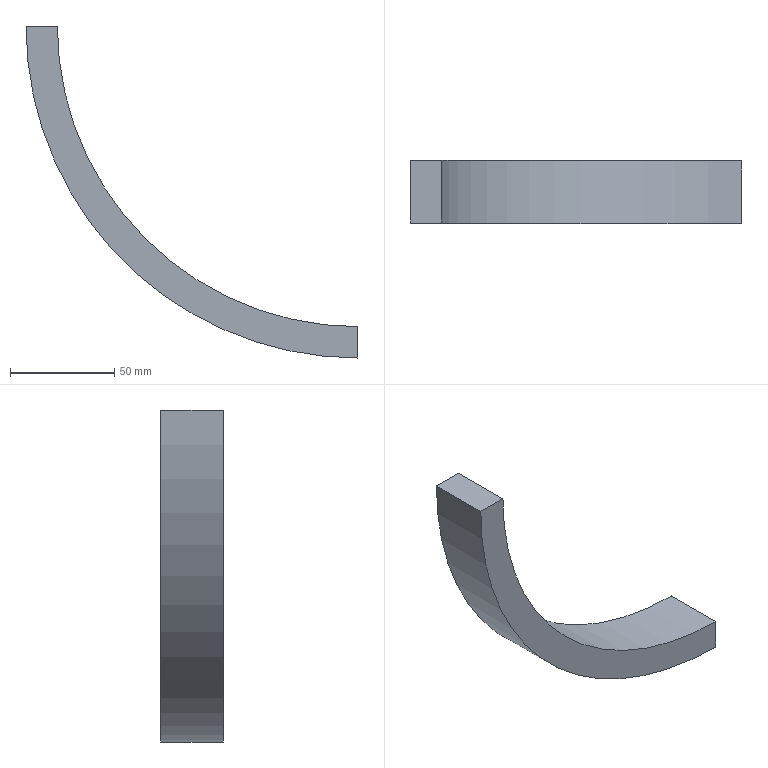Part | SolidWorks | features Extrusion 1 | 1 solid | 6 faces | box 159 x 30 x 159 mm | volume 107089 mm3 | plane 4 | cylinder 2 | commonest cylinder face diameters 288 x1 318 x1
STEP:
#1=CARTESIAN_POINT('',(-144.,0.,0.));
#2=VERTEX_POINT('',#1);
#3=CARTESIAN_POINT('',(0.,0.,-144.));
#4=VERTEX_POINT('',#3);
#5=CARTESIAN_POINT('',(0.,0.,0.));
#6=DIRECTION('',(0.,-1.,0.));
#7=DIRECTION('',(0.,0.,1.));
#8=AXIS2_PLACEMENT_3D('',#5,#6,#7);
#9=CIRCLE('',#8,144.);
#10=EDGE_CURVE('',#2,#4,#9,.T.);
#11=ORIENTED_EDGE('',*,*,#10,.T.);
#12=CARTESIAN_POINT('',(0.,30.,-144.));
#13=VERTEX_POINT('',#12);
#14=CARTESIAN_POINT('',(0.,30.,-144.));
#15=DIRECTION('',(0.,-1.,0.));
#16=VECTOR('',#15,1000.);
#17=LINE('',#14,#16);
#18=EDGE_CURVE('',#13,#4,#17,.T.);
#19=ORIENTED_EDGE('',*,*,#18,.F.);
#20=CARTESIAN_POINT('',(-144.,30.,0.));
#21=VERTEX_POINT('',#20);
#22=CARTESIAN_POINT('',(0.,30.,0.));
#23=DIRECTION('',(0.,-1.,0.));
#24=DIRECTION('',(0.,0.,1.));
#25=AXIS2_PLACEMENT_3D('',#22,#23,#24);
#26=CIRCLE('',#25,144.);
#27=EDGE_CURVE('',#21,#13,#26,.T.);
#28=ORIENTED_EDGE('',*,*,#27,.F.);
#29=CARTESIAN_POINT('',(-144.,30.,0.));
#30=DIRECTION('',(0.,-1.,0.));
#31=VECTOR('',#30,1000.);
#32=LINE('',#29,#31);
#33=EDGE_CURVE('',#21,#2,#32,.T.);
#34=ORIENTED_EDGE('',*,*,#33,.T.);
#35=EDGE_LOOP('',(#11,#19,#28,#34));
#36=FACE_OUTER_BOUND('',#35,.T.);
#37=CARTESIAN_POINT('',(0.,30.,0.));
#38=DIRECTION('',(0.,-1.,0.));
#39=DIRECTION('',(0.,0.,-1.));
#40=AXIS2_PLACEMENT_3D('',#37,#38,#39);
#41=CYLINDRICAL_SURFACE('',#40,144.);
#42=ADVANCED_FACE('',(#36),#41,.F.);
#43=CARTESIAN_POINT('',(0.,0.,-159.));
#44=VERTEX_POINT('',#43);
#45=CARTESIAN_POINT('',(0.,0.,-159.));
#46=DIRECTION('',(0.,0.,-1.));
#47=VECTOR('',#46,1000.);
#48=LINE('',#45,#47);
#49=EDGE_CURVE('',#4,#44,#48,.T.);
#50=ORIENTED_EDGE('',*,*,#49,.T.);
#51=CARTESIAN_POINT('',(0.,30.,-159.));
#52=VERTEX_POINT('',#51);
#53=CARTESIAN_POINT('',(0.,30.,-159.));
#54=DIRECTION('',(0.,-1.,0.));
#55=VECTOR('',#54,1000.);
#56=LINE('',#53,#55);
#57=EDGE_CURVE('',#52,#44,#56,.T.);
#58=ORIENTED_EDGE('',*,*,#57,.F.);
#59=CARTESIAN_POINT('',(0.,30.,-159.));
#60=DIRECTION('',(0.,0.,-1.));
#61=VECTOR('',#60,1000.);
#62=LINE('',#59,#61);
#63=EDGE_CURVE('',#13,#52,#62,.T.);
#64=ORIENTED_EDGE('',*,*,#63,.F.);
#65=ORIENTED_EDGE('',*,*,#18,.T.);
#66=EDGE_LOOP('',(#50,#58,#64,#65));
#67=FACE_OUTER_BOUND('',#66,.T.);
#68=CARTESIAN_POINT('',(0.,30.,-159.));
#69=DIRECTION('',(-1.,0.,0.));
#70=DIRECTION('',(0.,0.,1.));
#71=AXIS2_PLACEMENT_3D('',#68,#69,#70);
#72=PLANE('',#71);
#73=ADVANCED_FACE('',(#67),#72,.F.);
#74=CARTESIAN_POINT('',(-159.,0.,0.));
#75=VERTEX_POINT('',#74);
#76=CARTESIAN_POINT('',(0.,0.,0.));
#77=DIRECTION('',(0.,1.,0.));
#78=DIRECTION('',(0.,0.,1.));
#79=AXIS2_PLACEMENT_3D('',#76,#77,#78);
#80=CIRCLE('',#79,159.);
#81=EDGE_CURVE('',#44,#75,#80,.T.);
#82=ORIENTED_EDGE('',*,*,#81,.T.);
#83=CARTESIAN_POINT('',(-159.,30.,0.));
#84=VERTEX_POINT('',#83);
#85=CARTESIAN_POINT('',(-159.,30.,0.));
#86=DIRECTION('',(0.,-1.,0.));
#87=VECTOR('',#86,1000.);
#88=LINE('',#85,#87);
#89=EDGE_CURVE('',#84,#75,#88,.T.);
#90=ORIENTED_EDGE('',*,*,#89,.F.);
#91=CARTESIAN_POINT('',(0.,30.,0.));
#92=DIRECTION('',(0.,1.,0.));
#93=DIRECTION('',(0.,0.,1.));
#94=AXIS2_PLACEMENT_3D('',#91,#92,#93);
#95=CIRCLE('',#94,159.);
#96=EDGE_CURVE('',#52,#84,#95,.T.);
#97=ORIENTED_EDGE('',*,*,#96,.F.);
#98=ORIENTED_EDGE('',*,*,#57,.T.);
#99=EDGE_LOOP('',(#82,#90,#97,#98));
#100=FACE_OUTER_BOUND('',#99,.T.);
#101=CARTESIAN_POINT('',(0.,30.,0.));
#102=DIRECTION('',(0.,-1.,0.));
#103=DIRECTION('',(0.,0.,-1.));
#104=AXIS2_PLACEMENT_3D('',#101,#102,#103);
#105=CYLINDRICAL_SURFACE('',#104,159.);
#106=ADVANCED_FACE('',(#100),#105,.T.);
#107=CARTESIAN_POINT('',(-159.,0.,0.));
#108=DIRECTION('',(1.,0.,0.));
#109=VECTOR('',#108,1000.);
#110=LINE('',#107,#109);
#111=EDGE_CURVE('',#75,#2,#110,.T.);
#112=ORIENTED_EDGE('',*,*,#111,.T.);
#113=ORIENTED_EDGE('',*,*,#33,.F.);
#114=CARTESIAN_POINT('',(-159.,30.,0.));
#115=DIRECTION('',(1.,0.,0.));
#116=VECTOR('',#115,1000.);
#117=LINE('',#114,#116);
#118=EDGE_CURVE('',#84,#21,#117,.T.);
#119=ORIENTED_EDGE('',*,*,#118,.F.);
#120=ORIENTED_EDGE('',*,*,#89,.T.);
#121=EDGE_LOOP('',(#112,#113,#119,#120));
#122=FACE_OUTER_BOUND('',#121,.T.);
#123=CARTESIAN_POINT('',(-159.,30.,0.));
#124=DIRECTION('',(0.,0.,-1.));
#125=DIRECTION('',(-1.,0.,0.));
#126=AXIS2_PLACEMENT_3D('',#123,#124,#125);
#127=PLANE('',#126);
#128=ADVANCED_FACE('',(#122),#127,.F.);
#129=ORIENTED_EDGE('',*,*,#27,.T.);
#130=ORIENTED_EDGE('',*,*,#63,.T.);
#131=ORIENTED_EDGE('',*,*,#96,.T.);
#132=ORIENTED_EDGE('',*,*,#118,.T.);
#133=EDGE_LOOP('',(#129,#130,#131,#132));
#134=FACE_OUTER_BOUND('',#133,.T.);
#135=CARTESIAN_POINT('',(0.,30.,0.));
#136=DIRECTION('',(0.,1.,0.));
#137=DIRECTION('',(0.,0.,1.));
#138=AXIS2_PLACEMENT_3D('',#135,#136,#137);
#139=PLANE('',#138);
#140=ADVANCED_FACE('',(#134),#139,.T.);
#141=ORIENTED_EDGE('',*,*,#10,.F.);
#142=ORIENTED_EDGE('',*,*,#111,.F.);
#143=ORIENTED_EDGE('',*,*,#81,.F.);
#144=ORIENTED_EDGE('',*,*,#49,.F.);
#145=EDGE_LOOP('',(#141,#142,#143,#144));
#146=FACE_OUTER_BOUND('',#145,.T.);
#147=CARTESIAN_POINT('',(0.,0.,0.));
#148=DIRECTION('',(0.,1.,0.));
#149=DIRECTION('',(0.,0.,1.));
#150=AXIS2_PLACEMENT_3D('',#147,#148,#149);
#151=PLANE('',#150);
#152=ADVANCED_FACE('',(#146),#151,.F.);
#153=CLOSED_SHELL('',(#42,#73,#106,#128,#140,#152));
#154=MANIFOLD_SOLID_BREP('',#153);
#155=CARTESIAN_POINT('',(0.,0.,0.));
#156=DIRECTION('',(0.,0.,1.));
#157=DIRECTION('',(1.,0.,0.));
#158=AXIS2_PLACEMENT_3D('',#155,#156,#157);
#159=(LENGTH_UNIT()NAMED_UNIT(*)SI_UNIT(.MILLI.,.METRE.));
#160=UNCERTAINTY_MEASURE_WITH_UNIT(LENGTH_MEASURE(0.00001),#159,'','');
#161=(NAMED_UNIT(*)PLANE_ANGLE_UNIT()SI_UNIT($,.RADIAN.));
#162=(NAMED_UNIT(*)SI_UNIT($,.STERADIAN.)SOLID_ANGLE_UNIT());
#163=(GEOMETRIC_REPRESENTATION_CONTEXT(3)GLOBAL_UNCERTAINTY_ASSIGNED_CONTEXT((#160))GLOBAL_UNIT_ASSIGNED_CONTEXT((#159,#161,#162))REPRESENTATION_CONTEXT('',''));
#164=ADVANCED_BREP_SHAPE_REPRESENTATION('',(#154,#158),#163);